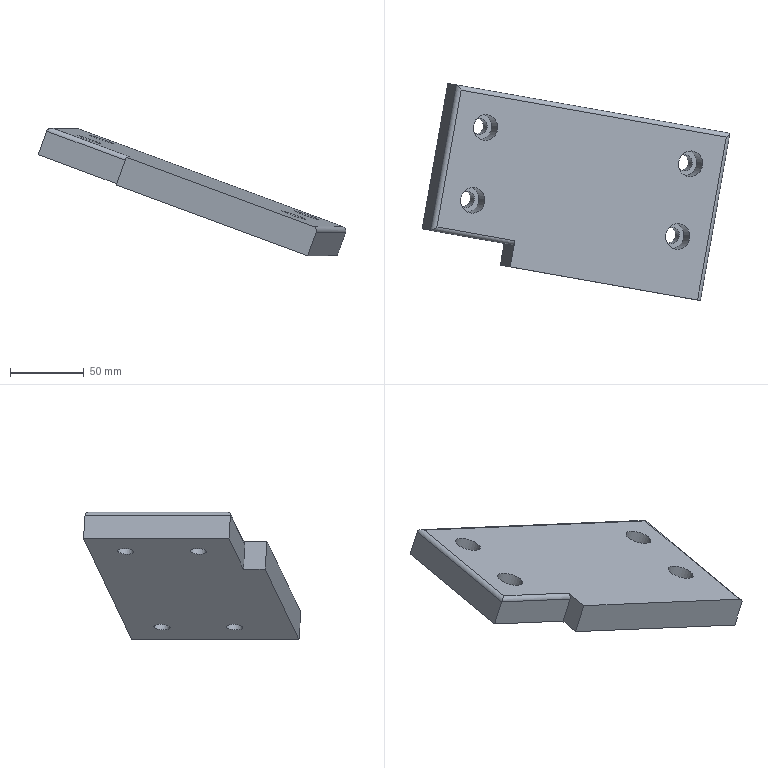Part | NX | features solid 2 | 1 solid | 24 faces | box 208.326 x 146.929 x 86.353 mm | volume 426504 mm3 | plane 12 | cylinder 12 | commonest cylinder face diameters 6 x4 11 x4 17.5 x4
STEP:
#1=CARTESIAN_POINT('',(-1087.888,-115.233,-183.949));
#2=VERTEX_POINT('',#1);
#3=CARTESIAN_POINT('',(-1143.413,-105.442,-163.428));
#4=VERTEX_POINT('',#3);
#5=CARTESIAN_POINT('',(-958.237,-138.094,-231.866));
#6=DIRECTION('',(-0.9254,0.1632,0.342));
#7=VECTOR('',#6,1000.);
#8=LINE('',#5,#7);
#9=EDGE_CURVE('',#2,#4,#8,.T.);
#10=ORIENTED_EDGE('',*,*,#9,.T.);
#11=CARTESIAN_POINT('',(-1149.139,-104.432,-179.402));
#12=VERTEX_POINT('',#11);
#13=CARTESIAN_POINT('',(-1142.369,-105.626,-160.515));
#14=DIRECTION('',(-0.3368,0.05939,-0.9397));
#15=VECTOR('',#14,1000.);
#16=LINE('',#13,#15);
#17=EDGE_CURVE('',#4,#12,#16,.T.);
#18=ORIENTED_EDGE('',*,*,#17,.T.);
#19=CARTESIAN_POINT('',(-1093.614,-114.223,-199.924));
#20=VERTEX_POINT('',#19);
#21=CARTESIAN_POINT('',(-963.871,-137.1,-247.875));
#22=DIRECTION('',(-0.9254,0.1632,0.342));
#23=VECTOR('',#22,1000.);
#24=LINE('',#21,#23);
#25=EDGE_CURVE('',#20,#12,#24,.T.);
#26=ORIENTED_EDGE('',*,*,#25,.F.);
#27=CARTESIAN_POINT('',(-1086.844,-115.417,-181.036));
#28=DIRECTION('',(-0.3368,0.05939,-0.9397));
#29=VECTOR('',#28,1000.);
#30=LINE('',#27,#29);
#31=EDGE_CURVE('',#2,#20,#30,.T.);
#32=ORIENTED_EDGE('',*,*,#31,.F.);
#33=EDGE_LOOP('',(#10,#18,#26,#32));
#34=FACE_BOUND('',#33,.T.);
#35=CARTESIAN_POINT('',(-957.193,-138.278,-228.953));
#36=DIRECTION('',(-0.1736,-0.9848,0.));
#37=DIRECTION('',(-0.9254,0.1632,0.342));
#38=AXIS2_PLACEMENT_3D('',#35,#36,#37);
#39=PLANE('',#38);
#40=ADVANCED_FACE('',(#34),#39,.T.);
#41=CARTESIAN_POINT('',(-940.965,-39.596,-231.832));
#42=VERTEX_POINT('',#41);
#43=CARTESIAN_POINT('',(-960.935,-152.849,-231.832));
#44=VERTEX_POINT('',#43);
#45=CARTESIAN_POINT('',(-959.016,-141.967,-231.832));
#46=DIRECTION('',(0.1736,0.9848,0.));
#47=VECTOR('',#46,1000.);
#48=LINE('',#45,#47);
#49=EDGE_CURVE('',#42,#44,#48,.F.);
#50=ORIENTED_EDGE('',*,*,#49,.F.);
#51=CARTESIAN_POINT('',(-943.252,-42.24,-227.987));
#52=VERTEX_POINT('',#51);
#53=CARTESIAN_POINT('',(-944.262,-42.061,-230.806));
#54=DIRECTION('',(-0.5316,0.8117,0.2418));
#55=DIRECTION('',(0.7772,0.581,-0.2418));
#56=AXIS2_PLACEMENT_3D('',#53,#54,#55);
#57=ELLIPSE('',#56,4.243,3.);
#58=EDGE_CURVE('',#52,#42,#57,.T.);
#59=ORIENTED_EDGE('',*,*,#58,.F.);
#60=CARTESIAN_POINT('',(-962.7,-152.538,-227.987));
#61=VERTEX_POINT('',#60);
#62=CARTESIAN_POINT('',(-940.543,-26.877,-227.987));
#63=DIRECTION('',(0.1736,0.9848,0.));
#64=VECTOR('',#63,1000.);
#65=LINE('',#62,#64);
#66=EDGE_CURVE('',#61,#52,#65,.T.);
#67=ORIENTED_EDGE('',*,*,#66,.F.);
#68=CARTESIAN_POINT('',(-963.711,-152.36,-230.806));
#69=DIRECTION('',(0.1736,0.9848,0.));
#70=DIRECTION('',(-0.9848,0.1736,0.));
#71=AXIS2_PLACEMENT_3D('',#68,#69,#70);
#72=CIRCLE('',#71,3.);
#73=EDGE_CURVE('',#44,#61,#72,.F.);
#74=ORIENTED_EDGE('',*,*,#73,.F.);
#75=EDGE_LOOP('',(#50,#59,#67,#74));
#76=FACE_BOUND('',#75,.T.);
#77=CARTESIAN_POINT('',(-941.553,-26.698,-230.806));
#78=DIRECTION('',(0.1736,0.9848,0.));
#79=DIRECTION('',(-0.9848,0.1736,0.));
#80=AXIS2_PLACEMENT_3D('',#77,#78,#79);
#81=CYLINDRICAL_SURFACE('',#80,3.);
#82=ADVANCED_FACE('',(#76),#81,.T.);
#83=CARTESIAN_POINT('',(-1139.105,-103.155,-161.635));
#84=VERTEX_POINT('',#83);
#85=CARTESIAN_POINT('',(-1086.357,-112.456,-181.13));
#86=VERTEX_POINT('',#85);
#87=CARTESIAN_POINT('',(-956.613,-135.334,-229.081));
#88=DIRECTION('',(-0.9254,0.1632,0.342));
#89=VECTOR('',#88,1000.);
#90=LINE('',#87,#89);
#91=EDGE_CURVE('',#84,#86,#90,.F.);
#92=ORIENTED_EDGE('',*,*,#91,.F.);
#93=CARTESIAN_POINT('',(-1140.116,-102.977,-164.454));
#94=DIRECTION('',(-0.5316,0.8117,0.2418));
#95=DIRECTION('',(-0.7772,-0.581,0.2418));
#96=AXIS2_PLACEMENT_3D('',#93,#94,#95);
#97=ELLIPSE('',#96,4.243,3.);
#98=EDGE_CURVE('',#4,#84,#97,.T.);
#99=ORIENTED_EDGE('',*,*,#98,.F.);
#100=ORIENTED_EDGE('',*,*,#9,.F.);
#101=CARTESIAN_POINT('',(-1087.367,-112.278,-183.949));
#102=DIRECTION('',(-0.9254,0.1632,0.342));
#103=DIRECTION('',(-0.3258,0.1186,-0.938));
#104=AXIS2_PLACEMENT_3D('',#101,#102,#103);
#105=CIRCLE('',#104,3.);
#106=EDGE_CURVE('',#86,#2,#105,.F.);
#107=ORIENTED_EDGE('',*,*,#106,.F.);
#108=EDGE_LOOP('',(#92,#99,#100,#107));
#109=FACE_BOUND('',#108,.T.);
#110=CARTESIAN_POINT('',(-957.716,-135.139,-231.866));
#111=DIRECTION('',(-0.9254,0.1632,0.342));
#112=DIRECTION('',(0.3368,-0.05939,0.9397));
#113=AXIS2_PLACEMENT_3D('',#110,#111,#112);
#114=CYLINDRICAL_SURFACE('',#113,3.);
#115=ADVANCED_FACE('',(#109),#114,.T.);
#116=CARTESIAN_POINT('',(-1089.482,-130.183,-181.13));
#117=VERTEX_POINT('',#116);
#118=CARTESIAN_POINT('',(-1086.878,-115.411,-181.13));
#119=DIRECTION('',(0.1736,0.9848,0.));
#120=VECTOR('',#119,1000.);
#121=LINE('',#118,#120);
#122=EDGE_CURVE('',#86,#117,#121,.F.);
#123=ORIENTED_EDGE('',*,*,#122,.T.);
#124=CARTESIAN_POINT('',(-959.832,-153.044,-229.047));
#125=DIRECTION('',(0.9254,-0.1632,-0.342));
#126=VECTOR('',#125,1000.);
#127=LINE('',#124,#126);
#128=EDGE_CURVE('',#61,#117,#127,.F.);
#129=ORIENTED_EDGE('',*,*,#128,.F.);
#130=ORIENTED_EDGE('',*,*,#66,.T.);
#131=CARTESIAN_POINT('',(-1122.783,-10.583,-161.635));
#132=VERTEX_POINT('',#131);
#133=CARTESIAN_POINT('',(-940.29,-42.762,-229.081));
#134=DIRECTION('',(-0.9254,0.1632,0.342));
#135=VECTOR('',#134,1000.);
#136=LINE('',#133,#135);
#137=EDGE_CURVE('',#52,#132,#136,.T.);
#138=ORIENTED_EDGE('',*,*,#137,.T.);
#139=CARTESIAN_POINT('',(-1120.074,4.78,-161.635));
#140=DIRECTION('',(0.1736,0.9848,0.));
#141=VECTOR('',#140,1000.);
#142=LINE('',#139,#141);
#143=EDGE_CURVE('',#132,#84,#142,.F.);
#144=ORIENTED_EDGE('',*,*,#143,.T.);
#145=ORIENTED_EDGE('',*,*,#91,.T.);
#146=EDGE_LOOP('',(#123,#129,#130,#138,#144,#145));
#147=FACE_BOUND('',#146,.T.);
#148=CARTESIAN_POINT('',(-975.529,-58.888,-217.469));
#149=VERTEX_POINT('',#148);
#150=CARTESIAN_POINT('',(-967.431,-60.315,-220.462));
#151=DIRECTION('',(-0.3368,0.05939,-0.9397));
#152=DIRECTION('',(-0.9254,0.1632,0.342));
#153=AXIS2_PLACEMENT_3D('',#150,#151,#152);
#154=CIRCLE('',#153,8.75);
#155=EDGE_CURVE('',#149,#149,#154,.T.);
#156=ORIENTED_EDGE('',*,*,#155,.T.);
#157=EDGE_LOOP('',(#156));
#158=FACE_BOUND('',#157,.T.);
#159=CARTESIAN_POINT('',(-984.211,-108.128,-217.469));
#160=VERTEX_POINT('',#159);
#161=CARTESIAN_POINT('',(-976.114,-109.556,-220.462));
#162=DIRECTION('',(-0.3368,0.05939,-0.9397));
#163=DIRECTION('',(-0.9254,0.1632,0.342));
#164=AXIS2_PLACEMENT_3D('',#161,#162,#163);
#165=CIRCLE('',#164,8.75);
#166=EDGE_CURVE('',#160,#160,#165,.T.);
#167=ORIENTED_EDGE('',*,*,#166,.T.);
#168=EDGE_LOOP('',(#167));
#169=FACE_BOUND('',#168,.T.);
#170=CARTESIAN_POINT('',(-1106.829,-86.507,-172.152));
#171=VERTEX_POINT('',#170);
#172=CARTESIAN_POINT('',(-1114.926,-85.079,-169.159));
#173=DIRECTION('',(0.3368,-0.05939,0.9397));
#174=DIRECTION('',(0.9254,-0.1632,-0.342));
#175=AXIS2_PLACEMENT_3D('',#172,#173,#174);
#176=CIRCLE('',#175,8.75);
#177=EDGE_CURVE('',#171,#171,#176,.F.);
#178=ORIENTED_EDGE('',*,*,#177,.T.);
#179=EDGE_LOOP('',(#178));
#180=FACE_BOUND('',#179,.T.);
#181=CARTESIAN_POINT('',(-1098.146,-37.267,-172.152));
#182=VERTEX_POINT('',#181);
#183=CARTESIAN_POINT('',(-1106.244,-35.839,-169.159));
#184=DIRECTION('',(0.3368,-0.05939,0.9397));
#185=DIRECTION('',(0.9254,-0.1632,-0.342));
#186=AXIS2_PLACEMENT_3D('',#183,#184,#185);
#187=CIRCLE('',#186,8.75);
#188=EDGE_CURVE('',#182,#182,#187,.F.);
#189=ORIENTED_EDGE('',*,*,#188,.T.);
#190=EDGE_LOOP('',(#189));
#191=FACE_BOUND('',#190,.T.);
#192=CARTESIAN_POINT('',(-937.581,-27.399,-229.081));
#193=DIRECTION('',(0.3368,-0.05939,0.9397));
#194=DIRECTION('',(-0.9254,0.1632,0.342));
#195=AXIS2_PLACEMENT_3D('',#192,#193,#194);
#196=PLANE('',#195);
#197=ADVANCED_FACE('',(#147,#158,#169,#180,#191),#196,.T.);
#198=CARTESIAN_POINT('',(-966.661,-151.84,-247.806));
#199=VERTEX_POINT('',#198);
#200=CARTESIAN_POINT('',(-959.89,-153.033,-228.919));
#201=DIRECTION('',(0.3368,-0.05939,0.9397));
#202=VECTOR('',#201,1000.);
#203=LINE('',#200,#202);
#204=EDGE_CURVE('',#199,#44,#203,.T.);
#205=ORIENTED_EDGE('',*,*,#204,.F.);
#206=CARTESIAN_POINT('',(-946.691,-38.587,-247.806));
#207=VERTEX_POINT('',#206);
#208=CARTESIAN_POINT('',(-944.52,-26.277,-247.806));
#209=DIRECTION('',(-0.1736,-0.9848,0.));
#210=VECTOR('',#209,1000.);
#211=LINE('',#208,#210);
#212=EDGE_CURVE('',#207,#199,#211,.T.);
#213=ORIENTED_EDGE('',*,*,#212,.F.);
#214=CARTESIAN_POINT('',(-947.062,-38.521,-248.84));
#215=DIRECTION('',(0.3368,-0.05939,0.9397));
#216=VECTOR('',#215,1000.);
#217=LINE('',#214,#216);
#218=EDGE_CURVE('',#207,#42,#217,.T.);
#219=ORIENTED_EDGE('',*,*,#218,.T.);
#220=ORIENTED_EDGE('',*,*,#49,.T.);
#221=EDGE_LOOP('',(#205,#213,#219,#220));
#222=FACE_BOUND('',#221,.T.);
#223=CARTESIAN_POINT('',(-965.112,-140.892,-248.84));
#224=DIRECTION('',(0.9254,-0.1632,-0.342));
#225=DIRECTION('',(0.1736,0.9848,0.));
#226=AXIS2_PLACEMENT_3D('',#223,#224,#225);
#227=PLANE('',#226);
#228=ADVANCED_FACE('',(#222),#227,.T.);
#229=ORIENTED_EDGE('',*,*,#25,.T.);
#230=CARTESIAN_POINT('',(-1131.774,-5.952,-179.402));
#231=VERTEX_POINT('',#230);
#232=CARTESIAN_POINT('',(-1146.812,-91.236,-179.402));
#233=DIRECTION('',(-0.1736,-0.9848,0.));
#234=VECTOR('',#233,1000.);
#235=LINE('',#232,#234);
#236=EDGE_CURVE('',#231,#12,#235,.T.);
#237=ORIENTED_EDGE('',*,*,#236,.F.);
#238=CARTESIAN_POINT('',(-946.506,-38.619,-247.875));
#239=DIRECTION('',(0.9254,-0.1632,-0.342));
#240=VECTOR('',#239,1000.);
#241=LINE('',#238,#240);
#242=EDGE_CURVE('',#231,#207,#241,.T.);
#243=ORIENTED_EDGE('',*,*,#242,.T.);
#244=ORIENTED_EDGE('',*,*,#212,.T.);
#245=CARTESIAN_POINT('',(-1096.219,-128.995,-199.924));
#246=VERTEX_POINT('',#245);
#247=CARTESIAN_POINT('',(-966.475,-151.872,-247.875));
#248=DIRECTION('',(-0.9254,0.1632,0.342));
#249=VECTOR('',#248,1000.);
#250=LINE('',#247,#249);
#251=EDGE_CURVE('',#199,#246,#250,.T.);
#252=ORIENTED_EDGE('',*,*,#251,.T.);
#253=CARTESIAN_POINT('',(-1093.614,-114.223,-199.924));
#254=DIRECTION('',(-0.1736,-0.9848,0.));
#255=VECTOR('',#254,1000.);
#256=LINE('',#253,#255);
#257=EDGE_CURVE('',#20,#246,#256,.T.);
#258=ORIENTED_EDGE('',*,*,#257,.F.);
#259=EDGE_LOOP('',(#229,#237,#243,#244,#252,#258));
#260=FACE_BOUND('',#259,.T.);
#261=CARTESIAN_POINT('',(-979.257,-58.23,-237.375));
#262=VERTEX_POINT('',#261);
#263=CARTESIAN_POINT('',(-974.168,-59.128,-239.256));
#264=DIRECTION('',(-0.3368,0.05939,-0.9397));
#265=DIRECTION('',(-0.9254,0.1632,0.342));
#266=AXIS2_PLACEMENT_3D('',#263,#264,#265);
#267=CIRCLE('',#266,5.5);
#268=EDGE_CURVE('',#262,#262,#267,.T.);
#269=ORIENTED_EDGE('',*,*,#268,.F.);
#270=EDGE_LOOP('',(#269));
#271=FACE_BOUND('',#270,.T.);
#272=CARTESIAN_POINT('',(-987.94,-107.471,-237.375));
#273=VERTEX_POINT('',#272);
#274=CARTESIAN_POINT('',(-982.85,-108.368,-239.256));
#275=DIRECTION('',(-0.3368,0.05939,-0.9397));
#276=DIRECTION('',(-0.9254,0.1632,0.342));
#277=AXIS2_PLACEMENT_3D('',#274,#275,#276);
#278=CIRCLE('',#277,5.5);
#279=EDGE_CURVE('',#273,#273,#278,.T.);
#280=ORIENTED_EDGE('',*,*,#279,.F.);
#281=EDGE_LOOP('',(#280));
#282=FACE_BOUND('',#281,.T.);
#283=CARTESIAN_POINT('',(-1126.752,-82.994,-186.072));
#284=VERTEX_POINT('',#283);
#285=CARTESIAN_POINT('',(-1121.663,-83.892,-187.953));
#286=DIRECTION('',(-0.3368,0.05939,-0.9397));
#287=DIRECTION('',(-0.9254,0.1632,0.342));
#288=AXIS2_PLACEMENT_3D('',#285,#286,#287);
#289=CIRCLE('',#288,5.5);
#290=EDGE_CURVE('',#284,#284,#289,.T.);
#291=ORIENTED_EDGE('',*,*,#290,.F.);
#292=EDGE_LOOP('',(#291));
#293=FACE_BOUND('',#292,.T.);
#294=CARTESIAN_POINT('',(-1118.07,-33.754,-186.072));
#295=VERTEX_POINT('',#294);
#296=CARTESIAN_POINT('',(-1112.98,-34.651,-187.953));
#297=DIRECTION('',(-0.3368,0.05939,-0.9397));
#298=DIRECTION('',(-0.9254,0.1632,0.342));
#299=AXIS2_PLACEMENT_3D('',#296,#297,#298);
#300=CIRCLE('',#299,5.5);
#301=EDGE_CURVE('',#295,#295,#300,.T.);
#302=ORIENTED_EDGE('',*,*,#301,.F.);
#303=EDGE_LOOP('',(#302));
#304=FACE_BOUND('',#303,.T.);
#305=CARTESIAN_POINT('',(-964.574,-141.089,-247.875));
#306=DIRECTION('',(-0.3368,0.05939,-0.9397));
#307=DIRECTION('',(-0.9254,0.1632,0.342));
#308=AXIS2_PLACEMENT_3D('',#305,#306,#307);
#309=PLANE('',#308);
#310=ADVANCED_FACE('',(#260,#271,#282,#293,#304),#309,.T.);
#311=ORIENTED_EDGE('',*,*,#17,.F.);
#312=CARTESIAN_POINT('',(-1126.048,-6.961,-163.428));
#313=VERTEX_POINT('',#312);
#314=CARTESIAN_POINT('',(-1141.086,-92.246,-163.428));
#315=DIRECTION('',(0.1736,0.9848,0.));
#316=VECTOR('',#315,1000.);
#317=LINE('',#314,#316);
#318=EDGE_CURVE('',#4,#313,#317,.T.);
#319=ORIENTED_EDGE('',*,*,#318,.T.);
#320=CARTESIAN_POINT('',(-1125.004,-7.145,-160.515));
#321=DIRECTION('',(-0.3368,0.05939,-0.9397));
#322=VECTOR('',#321,1000.);
#323=LINE('',#320,#322);
#324=EDGE_CURVE('',#313,#231,#323,.T.);
#325=ORIENTED_EDGE('',*,*,#324,.T.);
#326=ORIENTED_EDGE('',*,*,#236,.T.);
#327=EDGE_LOOP('',(#311,#319,#325,#326));
#328=FACE_BOUND('',#327,.T.);
#329=CARTESIAN_POINT('',(-1140.042,-92.43,-160.515));
#330=DIRECTION('',(-0.9254,0.1632,0.342));
#331=DIRECTION('',(0.1736,0.9848,0.));
#332=AXIS2_PLACEMENT_3D('',#329,#330,#331);
#333=PLANE('',#332);
#334=ADVANCED_FACE('',(#328),#333,.T.);
#335=ORIENTED_EDGE('',*,*,#324,.F.);
#336=CARTESIAN_POINT('',(-934.024,-40.82,-234.397));
#337=DIRECTION('',(-0.9254,0.1632,0.342));
#338=VECTOR('',#337,1000.);
#339=LINE('',#336,#338);
#340=EDGE_CURVE('',#313,#42,#339,.F.);
#341=ORIENTED_EDGE('',*,*,#340,.T.);
#342=ORIENTED_EDGE('',*,*,#218,.F.);
#343=ORIENTED_EDGE('',*,*,#242,.F.);
#344=EDGE_LOOP('',(#335,#341,#342,#343));
#345=FACE_BOUND('',#344,.T.);
#346=CARTESIAN_POINT('',(-940.087,-39.751,-251.311));
#347=DIRECTION('',(0.1736,0.9848,0.));
#348=DIRECTION('',(-0.9254,0.1632,0.342));
#349=AXIS2_PLACEMENT_3D('',#346,#347,#348);
#350=PLANE('',#349);
#351=ADVANCED_FACE('',(#345),#350,.T.);
#352=ORIENTED_EDGE('',*,*,#268,.T.);
#353=EDGE_LOOP('',(#352));
#354=FACE_BOUND('',#353,.T.);
#355=CARTESIAN_POINT('',(-976.563,-58.705,-229.857));
#356=VERTEX_POINT('',#355);
#357=CARTESIAN_POINT('',(-971.473,-59.603,-231.738));
#358=DIRECTION('',(-0.3368,0.05939,-0.9397));
#359=DIRECTION('',(-0.9254,0.1632,0.342));
#360=AXIS2_PLACEMENT_3D('',#357,#358,#359);
#361=CIRCLE('',#360,5.5);
#362=EDGE_CURVE('',#356,#356,#361,.T.);
#363=ORIENTED_EDGE('',*,*,#362,.F.);
#364=EDGE_LOOP('',(#363));
#365=FACE_BOUND('',#364,.T.);
#366=CARTESIAN_POINT('',(-984.272,-57.346,-267.447));
#367=DIRECTION('',(-0.3368,0.05939,-0.9397));
#368=DIRECTION('',(-0.9254,0.1632,0.342));
#369=AXIS2_PLACEMENT_3D('',#366,#367,#368);
#370=CYLINDRICAL_SURFACE('',#369,5.5);
#371=ADVANCED_FACE('',(#354,#365),#370,.F.);
#372=ORIENTED_EDGE('',*,*,#362,.T.);
#373=EDGE_LOOP('',(#372));
#374=FACE_BOUND('',#373,.T.);
#375=CARTESIAN_POINT('',(-979.57,-58.175,-228.746));
#376=VERTEX_POINT('',#375);
#377=CARTESIAN_POINT('',(-971.473,-59.603,-231.738));
#378=DIRECTION('',(-0.3368,0.05939,-0.9397));
#379=DIRECTION('',(-0.9254,0.1632,0.342));
#380=AXIS2_PLACEMENT_3D('',#377,#378,#379);
#381=CIRCLE('',#380,8.75);
#382=EDGE_CURVE('',#376,#376,#381,.T.);
#383=ORIENTED_EDGE('',*,*,#382,.F.);
#384=EDGE_LOOP('',(#383));
#385=FACE_BOUND('',#384,.T.);
#386=CARTESIAN_POINT('',(-973.557,-71.42,-231.738));
#387=DIRECTION('',(-0.3368,0.05939,-0.9397));
#388=DIRECTION('',(-0.9254,0.1632,0.342));
#389=AXIS2_PLACEMENT_3D('',#386,#387,#388);
#390=PLANE('',#389);
#391=ADVANCED_FACE('',(#374,#385),#390,.F.);
#392=ORIENTED_EDGE('',*,*,#382,.T.);
#393=EDGE_LOOP('',(#392));
#394=FACE_BOUND('',#393,.T.);
#395=ORIENTED_EDGE('',*,*,#155,.F.);
#396=EDGE_LOOP('',(#395));
#397=FACE_BOUND('',#396,.T.);
#398=CARTESIAN_POINT('',(-967.431,-60.315,-220.462));
#399=DIRECTION('',(-0.3368,0.05939,-0.9397));
#400=DIRECTION('',(-0.9254,0.1632,0.342));
#401=AXIS2_PLACEMENT_3D('',#398,#399,#400);
#402=CYLINDRICAL_SURFACE('',#401,8.75);
#403=ADVANCED_FACE('',(#394,#397),#402,.F.);
#404=ORIENTED_EDGE('',*,*,#279,.T.);
#405=EDGE_LOOP('',(#404));
#406=FACE_BOUND('',#405,.T.);
#407=CARTESIAN_POINT('',(-985.245,-107.946,-229.857));
#408=VERTEX_POINT('',#407);
#409=CARTESIAN_POINT('',(-980.155,-108.843,-231.738));
#410=DIRECTION('',(-0.3368,0.05939,-0.9397));
#411=DIRECTION('',(-0.9254,0.1632,0.342));
#412=AXIS2_PLACEMENT_3D('',#409,#410,#411);
#413=CIRCLE('',#412,5.5);
#414=EDGE_CURVE('',#408,#408,#413,.T.);
#415=ORIENTED_EDGE('',*,*,#414,.F.);
#416=EDGE_LOOP('',(#415));
#417=FACE_BOUND('',#416,.T.);
#418=CARTESIAN_POINT('',(-992.955,-106.586,-267.447));
#419=DIRECTION('',(-0.3368,0.05939,-0.9397));
#420=DIRECTION('',(-0.9254,0.1632,0.342));
#421=AXIS2_PLACEMENT_3D('',#418,#419,#420);
#422=CYLINDRICAL_SURFACE('',#421,5.5);
#423=ADVANCED_FACE('',(#406,#417),#422,.F.);
#424=ORIENTED_EDGE('',*,*,#414,.T.);
#425=EDGE_LOOP('',(#424));
#426=FACE_BOUND('',#425,.T.);
#427=CARTESIAN_POINT('',(-988.253,-107.415,-228.746));
#428=VERTEX_POINT('',#427);
#429=CARTESIAN_POINT('',(-980.155,-108.843,-231.738));
#430=DIRECTION('',(-0.3368,0.05939,-0.9397));
#431=DIRECTION('',(-0.9254,0.1632,0.342));
#432=AXIS2_PLACEMENT_3D('',#429,#430,#431);
#433=CIRCLE('',#432,8.75);
#434=EDGE_CURVE('',#428,#428,#433,.T.);
#435=ORIENTED_EDGE('',*,*,#434,.F.);
#436=EDGE_LOOP('',(#435));
#437=FACE_BOUND('',#436,.T.);
#438=CARTESIAN_POINT('',(-977.898,-96.041,-231.738));
#439=DIRECTION('',(-0.3368,0.05939,-0.9397));
#440=DIRECTION('',(-0.9254,0.1632,0.342));
#441=AXIS2_PLACEMENT_3D('',#438,#439,#440);
#442=PLANE('',#441);
#443=ADVANCED_FACE('',(#426,#437),#442,.F.);
#444=ORIENTED_EDGE('',*,*,#434,.T.);
#445=EDGE_LOOP('',(#444));
#446=FACE_BOUND('',#445,.T.);
#447=ORIENTED_EDGE('',*,*,#166,.F.);
#448=EDGE_LOOP('',(#447));
#449=FACE_BOUND('',#448,.T.);
#450=CARTESIAN_POINT('',(-976.114,-109.556,-220.462));
#451=DIRECTION('',(-0.3368,0.05939,-0.9397));
#452=DIRECTION('',(-0.9254,0.1632,0.342));
#453=AXIS2_PLACEMENT_3D('',#450,#451,#452);
#454=CYLINDRICAL_SURFACE('',#453,8.75);
#455=ADVANCED_FACE('',(#446,#449),#454,.F.);
#456=ORIENTED_EDGE('',*,*,#290,.T.);
#457=EDGE_LOOP('',(#456));
#458=FACE_BOUND('',#457,.T.);
#459=CARTESIAN_POINT('',(-1124.058,-83.469,-178.554));
#460=VERTEX_POINT('',#459);
#461=CARTESIAN_POINT('',(-1118.968,-84.367,-180.435));
#462=DIRECTION('',(-0.3368,0.05939,-0.9397));
#463=DIRECTION('',(-0.9254,0.1632,0.342));
#464=AXIS2_PLACEMENT_3D('',#461,#462,#463);
#465=CIRCLE('',#464,5.5);
#466=EDGE_CURVE('',#460,#460,#465,.T.);
#467=ORIENTED_EDGE('',*,*,#466,.F.);
#468=EDGE_LOOP('',(#467));
#469=FACE_BOUND('',#468,.T.);
#470=CARTESIAN_POINT('',(-1131.767,-82.11,-216.144));
#471=DIRECTION('',(-0.3368,0.05939,-0.9397));
#472=DIRECTION('',(-0.9254,0.1632,0.342));
#473=AXIS2_PLACEMENT_3D('',#470,#471,#472);
#474=CYLINDRICAL_SURFACE('',#473,5.5);
#475=ADVANCED_FACE('',(#458,#469),#474,.F.);
#476=ORIENTED_EDGE('',*,*,#466,.T.);
#477=EDGE_LOOP('',(#476));
#478=FACE_BOUND('',#477,.T.);
#479=CARTESIAN_POINT('',(-1127.065,-82.939,-177.443));
#480=VERTEX_POINT('',#479);
#481=CARTESIAN_POINT('',(-1118.968,-84.367,-180.435));
#482=DIRECTION('',(-0.3368,0.05939,-0.9397));
#483=DIRECTION('',(-0.9254,0.1632,0.342));
#484=AXIS2_PLACEMENT_3D('',#481,#482,#483);
#485=CIRCLE('',#484,8.75);
#486=EDGE_CURVE('',#480,#480,#485,.T.);
#487=ORIENTED_EDGE('',*,*,#486,.F.);
#488=EDGE_LOOP('',(#487));
#489=FACE_BOUND('',#488,.T.);
#490=CARTESIAN_POINT('',(-1162.981,-63.405,-163.334));
#491=DIRECTION('',(-0.3368,0.05939,-0.9397));
#492=DIRECTION('',(-0.9254,0.1632,0.342));
#493=AXIS2_PLACEMENT_3D('',#490,#491,#492);
#494=PLANE('',#493);
#495=ADVANCED_FACE('',(#478,#489),#494,.F.);
#496=ORIENTED_EDGE('',*,*,#486,.T.);
#497=EDGE_LOOP('',(#496));
#498=FACE_BOUND('',#497,.T.);
#499=ORIENTED_EDGE('',*,*,#177,.F.);
#500=EDGE_LOOP('',(#499));
#501=FACE_BOUND('',#500,.T.);
#502=CARTESIAN_POINT('',(-1114.926,-85.079,-169.159));
#503=DIRECTION('',(-0.3368,0.05939,-0.9397));
#504=DIRECTION('',(-0.9254,0.1632,0.342));
#505=AXIS2_PLACEMENT_3D('',#502,#503,#504);
#506=CYLINDRICAL_SURFACE('',#505,8.75);
#507=ADVANCED_FACE('',(#498,#501),#506,.F.);
#508=ORIENTED_EDGE('',*,*,#301,.T.);
#509=EDGE_LOOP('',(#508));
#510=FACE_BOUND('',#509,.T.);
#511=CARTESIAN_POINT('',(-1115.375,-34.229,-178.554));
#512=VERTEX_POINT('',#511);
#513=CARTESIAN_POINT('',(-1110.286,-35.126,-180.435));
#514=DIRECTION('',(-0.3368,0.05939,-0.9397));
#515=DIRECTION('',(-0.9254,0.1632,0.342));
#516=AXIS2_PLACEMENT_3D('',#513,#514,#515);
#517=CIRCLE('',#516,5.5);
#518=EDGE_CURVE('',#512,#512,#517,.T.);
#519=ORIENTED_EDGE('',*,*,#518,.F.);
#520=EDGE_LOOP('',(#519));
#521=FACE_BOUND('',#520,.T.);
#522=CARTESIAN_POINT('',(-1123.085,-32.869,-216.144));
#523=DIRECTION('',(-0.3368,0.05939,-0.9397));
#524=DIRECTION('',(-0.9254,0.1632,0.342));
#525=AXIS2_PLACEMENT_3D('',#522,#523,#524);
#526=CYLINDRICAL_SURFACE('',#525,5.5);
#527=ADVANCED_FACE('',(#510,#521),#526,.F.);
#528=ORIENTED_EDGE('',*,*,#518,.T.);
#529=EDGE_LOOP('',(#528));
#530=FACE_BOUND('',#529,.T.);
#531=CARTESIAN_POINT('',(-1118.383,-33.699,-177.443));
#532=VERTEX_POINT('',#531);
#533=CARTESIAN_POINT('',(-1110.286,-35.126,-180.435));
#534=DIRECTION('',(-0.3368,0.05939,-0.9397));
#535=DIRECTION('',(-0.9254,0.1632,0.342));
#536=AXIS2_PLACEMENT_3D('',#533,#534,#535);
#537=CIRCLE('',#536,8.75);
#538=EDGE_CURVE('',#532,#532,#537,.T.);
#539=ORIENTED_EDGE('',*,*,#538,.F.);
#540=EDGE_LOOP('',(#539));
#541=FACE_BOUND('',#540,.T.);
#542=CARTESIAN_POINT('',(-1112.369,-46.944,-180.435));
#543=DIRECTION('',(-0.3368,0.05939,-0.9397));
#544=DIRECTION('',(-0.9254,0.1632,0.342));
#545=AXIS2_PLACEMENT_3D('',#542,#543,#544);
#546=PLANE('',#545);
#547=ADVANCED_FACE('',(#530,#541),#546,.F.);
#548=ORIENTED_EDGE('',*,*,#538,.T.);
#549=EDGE_LOOP('',(#548));
#550=FACE_BOUND('',#549,.T.);
#551=ORIENTED_EDGE('',*,*,#188,.F.);
#552=EDGE_LOOP('',(#551));
#553=FACE_BOUND('',#552,.T.);
#554=CARTESIAN_POINT('',(-1106.244,-35.839,-169.159));
#555=DIRECTION('',(-0.3368,0.05939,-0.9397));
#556=DIRECTION('',(-0.9254,0.1632,0.342));
#557=AXIS2_PLACEMENT_3D('',#554,#555,#556);
#558=CYLINDRICAL_SURFACE('',#557,8.75);
#559=ADVANCED_FACE('',(#550,#553),#558,.F.);
#560=ORIENTED_EDGE('',*,*,#58,.T.);
#561=ORIENTED_EDGE('',*,*,#340,.F.);
#562=CARTESIAN_POINT('',(-1123.793,-10.405,-164.454));
#563=DIRECTION('',(-0.7772,-0.581,0.2418));
#564=DIRECTION('',(-0.5316,0.8117,0.2418));
#565=AXIS2_PLACEMENT_3D('',#562,#563,#564);
#566=ELLIPSE('',#565,4.243,3.);
#567=EDGE_CURVE('',#132,#313,#566,.T.);
#568=ORIENTED_EDGE('',*,*,#567,.F.);
#569=ORIENTED_EDGE('',*,*,#137,.F.);
#570=EDGE_LOOP('',(#560,#561,#568,#569));
#571=FACE_BOUND('',#570,.T.);
#572=CARTESIAN_POINT('',(-941.301,-42.583,-231.9));
#573=DIRECTION('',(-0.9254,0.1632,0.342));
#574=DIRECTION('',(0.3368,-0.05939,0.9397));
#575=AXIS2_PLACEMENT_3D('',#572,#573,#574);
#576=CYLINDRICAL_SURFACE('',#575,3.);
#577=ADVANCED_FACE('',(#571),#576,.T.);
#578=ORIENTED_EDGE('',*,*,#98,.T.);
#579=ORIENTED_EDGE('',*,*,#143,.F.);
#580=ORIENTED_EDGE('',*,*,#567,.T.);
#581=ORIENTED_EDGE('',*,*,#318,.F.);
#582=EDGE_LOOP('',(#578,#579,#580,#581));
#583=FACE_BOUND('',#582,.T.);
#584=CARTESIAN_POINT('',(-1138.31,-92.735,-164.454));
#585=DIRECTION('',(0.1736,0.9848,0.));
#586=DIRECTION('',(-0.9848,0.1736,0.));
#587=AXIS2_PLACEMENT_3D('',#584,#585,#586);
#588=CYLINDRICAL_SURFACE('',#587,3.);
#589=ADVANCED_FACE('',(#583),#588,.T.);
#590=ORIENTED_EDGE('',*,*,#31,.T.);
#591=ORIENTED_EDGE('',*,*,#257,.T.);
#592=CARTESIAN_POINT('',(-1089.449,-130.189,-181.036));
#593=DIRECTION('',(-0.3368,0.05939,-0.9397));
#594=VECTOR('',#593,1000.);
#595=LINE('',#592,#594);
#596=EDGE_CURVE('',#117,#246,#595,.T.);
#597=ORIENTED_EDGE('',*,*,#596,.F.);
#598=ORIENTED_EDGE('',*,*,#122,.F.);
#599=ORIENTED_EDGE('',*,*,#106,.T.);
#600=EDGE_LOOP('',(#590,#591,#597,#598,#599));
#601=FACE_BOUND('',#600,.T.);
#602=CARTESIAN_POINT('',(-1086.844,-115.417,-181.036));
#603=DIRECTION('',(0.9254,-0.1632,-0.342));
#604=DIRECTION('',(-0.3258,0.1186,-0.938));
#605=AXIS2_PLACEMENT_3D('',#602,#603,#604);
#606=PLANE('',#605);
#607=ADVANCED_FACE('',(#601),#606,.F.);
#608=ORIENTED_EDGE('',*,*,#73,.T.);
#609=ORIENTED_EDGE('',*,*,#128,.T.);
#610=ORIENTED_EDGE('',*,*,#596,.T.);
#611=ORIENTED_EDGE('',*,*,#251,.F.);
#612=ORIENTED_EDGE('',*,*,#204,.T.);
#613=EDGE_LOOP('',(#608,#609,#610,#611,#612));
#614=FACE_BOUND('',#613,.T.);
#615=CARTESIAN_POINT('',(-959.798,-153.05,-228.953));
#616=DIRECTION('',(-0.1736,-0.9848,0.));
#617=DIRECTION('',(-0.9254,0.1632,0.342));
#618=AXIS2_PLACEMENT_3D('',#615,#616,#617);
#619=PLANE('',#618);
#620=ADVANCED_FACE('',(#614),#619,.T.);
#621=CLOSED_SHELL('',(#40,#82,#115,#197,#228,#310,#334,#351,#371,#391,#403,#423,#443,#455,#475,#495,#507,#527,#547,#559,#577,#589,#607,#620));
#622=MANIFOLD_SOLID_BREP('',#621);
#623=(LENGTH_UNIT()NAMED_UNIT(*)SI_UNIT(.MILLI.,.METRE.));
#624=UNCERTAINTY_MEASURE_WITH_UNIT(LENGTH_MEASURE(0.00001),#623,'','');
#625=(NAMED_UNIT(*)PLANE_ANGLE_UNIT()SI_UNIT($,.RADIAN.));
#626=(NAMED_UNIT(*)SI_UNIT($,.STERADIAN.)SOLID_ANGLE_UNIT());
#627=(GEOMETRIC_REPRESENTATION_CONTEXT(3)GLOBAL_UNCERTAINTY_ASSIGNED_CONTEXT((#624))GLOBAL_UNIT_ASSIGNED_CONTEXT((#623,#625,#626))REPRESENTATION_CONTEXT('',''));
#628=ADVANCED_BREP_SHAPE_REPRESENTATION('',(#622),#627);